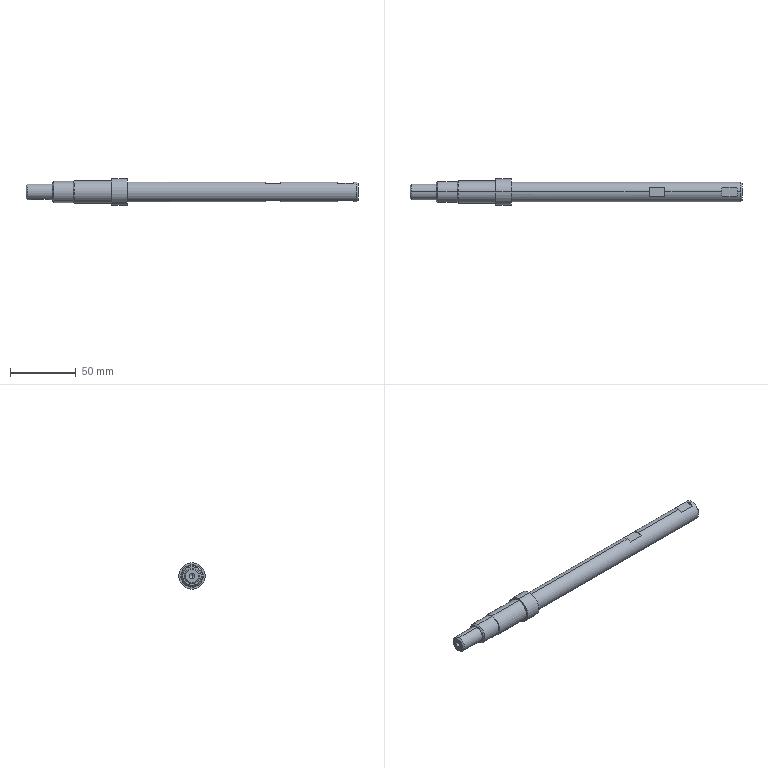Part | STEP file | MT-COMBO-119-S046 | 1 solid | 49 faces | box 252 x 20 x 20 mm | volume 45952 mm3 | plane 20 | cylinder 17 | cone 12 | commonest cylinder face diameters 4.2 x4 4 x3 12 x2 15 x2 16 x2 17 x2
STEP:
#1=CARTESIAN_POINT('',(-216.,0.,-8.));
#2=VERTEX_POINT('',#1);
#3=CARTESIAN_POINT('',(-216.,0.,8.));
#4=VERTEX_POINT('',#3);
#5=CARTESIAN_POINT('',(-216.,0.,0.));
#6=DIRECTION('',(1.,0.,0.));
#7=DIRECTION('',(0.,0.,-1.));
#8=AXIS2_PLACEMENT_3D('',#5,#6,#7);
#9=CIRCLE('',#8,8.);
#10=EDGE_CURVE('',#2,#4,#9,.T.);
#11=ORIENTED_EDGE('',*,*,#10,.T.);
#12=CARTESIAN_POINT('',(-215.5,0.,8.5));
#13=VERTEX_POINT('',#12);
#14=CARTESIAN_POINT('',(-215.5,0.,8.5));
#15=DIRECTION('',(0.7071,0.,0.7071));
#16=VECTOR('',#15,1000.);
#17=LINE('',#14,#16);
#18=EDGE_CURVE('',#4,#13,#17,.T.);
#19=ORIENTED_EDGE('',*,*,#18,.T.);
#20=CARTESIAN_POINT('',(-215.5,0.,-8.5));
#21=VERTEX_POINT('',#20);
#22=CARTESIAN_POINT('',(-215.5,0.,0.));
#23=DIRECTION('',(1.,0.,0.));
#24=DIRECTION('',(0.,0.,1.));
#25=AXIS2_PLACEMENT_3D('',#22,#23,#24);
#26=CIRCLE('',#25,8.5);
#27=EDGE_CURVE('',#21,#13,#26,.T.);
#28=ORIENTED_EDGE('',*,*,#27,.F.);
#29=CARTESIAN_POINT('',(-215.5,0.,-8.5));
#30=DIRECTION('',(0.7071,0.,-0.7071));
#31=VECTOR('',#30,1000.);
#32=LINE('',#29,#31);
#33=EDGE_CURVE('',#2,#21,#32,.T.);
#34=ORIENTED_EDGE('',*,*,#33,.F.);
#35=EDGE_LOOP('',(#11,#19,#28,#34));
#36=FACE_OUTER_BOUND('',#35,.T.);
#37=CARTESIAN_POINT('',(-215.5,0.,0.));
#38=DIRECTION('',(1.,0.,0.));
#39=DIRECTION('',(0.,0.,-1.));
#40=AXIS2_PLACEMENT_3D('',#37,#38,#39);
#41=CONICAL_SURFACE('',#40,8.5,0.7854);
#42=ADVANCED_FACE('',(#36),#41,.T.);
#43=CARTESIAN_POINT('',(-232.,0.,7.));
#44=VERTEX_POINT('',#43);
#45=CARTESIAN_POINT('',(-232.,0.,-7.));
#46=VERTEX_POINT('',#45);
#47=CARTESIAN_POINT('',(-232.,0.,0.));
#48=DIRECTION('',(-1.,0.,0.));
#49=DIRECTION('',(0.,0.,1.));
#50=AXIS2_PLACEMENT_3D('',#47,#48,#49);
#51=CIRCLE('',#50,7.);
#52=EDGE_CURVE('',#44,#46,#51,.T.);
#53=ORIENTED_EDGE('',*,*,#52,.F.);
#54=CARTESIAN_POINT('',(-231.,0.,8.));
#55=VERTEX_POINT('',#54);
#56=CARTESIAN_POINT('',(-231.,0.,8.));
#57=DIRECTION('',(0.7071,0.,0.7071));
#58=VECTOR('',#57,1000.);
#59=LINE('',#56,#58);
#60=EDGE_CURVE('',#44,#55,#59,.T.);
#61=ORIENTED_EDGE('',*,*,#60,.T.);
#62=CARTESIAN_POINT('',(-231.,0.,-8.));
#63=VERTEX_POINT('',#62);
#64=CARTESIAN_POINT('',(-231.,0.,0.));
#65=DIRECTION('',(1.,0.,0.));
#66=DIRECTION('',(0.,0.,1.));
#67=AXIS2_PLACEMENT_3D('',#64,#65,#66);
#68=CIRCLE('',#67,8.);
#69=EDGE_CURVE('',#63,#55,#68,.T.);
#70=ORIENTED_EDGE('',*,*,#69,.F.);
#71=CARTESIAN_POINT('',(-231.,0.,-8.));
#72=DIRECTION('',(0.7071,0.,-0.7071));
#73=VECTOR('',#72,1000.);
#74=LINE('',#71,#73);
#75=EDGE_CURVE('',#46,#63,#74,.T.);
#76=ORIENTED_EDGE('',*,*,#75,.F.);
#77=EDGE_LOOP('',(#53,#61,#70,#76));
#78=FACE_OUTER_BOUND('',#77,.T.);
#79=CARTESIAN_POINT('',(-231.,0.,0.));
#80=DIRECTION('',(1.,0.,0.));
#81=DIRECTION('',(0.,0.,-1.));
#82=AXIS2_PLACEMENT_3D('',#79,#80,#81);
#83=CONICAL_SURFACE('',#82,8.,0.7854);
#84=ADVANCED_FACE('',(#78),#83,.T.);
#85=CARTESIAN_POINT('',(-236.,2.,-5.657));
#86=VERTEX_POINT('',#85);
#87=CARTESIAN_POINT('',(-234.,0.,-6.));
#88=VERTEX_POINT('',#87);
#89=CARTESIAN_POINT('',(-236.,2.,-5.657));
#90=CARTESIAN_POINT('',(-235.867,2.,-5.657));
#91=CARTESIAN_POINT('',(-235.736,1.987,-5.662));
#92=CARTESIAN_POINT('',(-235.479,1.935,-5.679));
#93=CARTESIAN_POINT('',(-235.351,1.896,-5.693));
#94=CARTESIAN_POINT('',(-235.11,1.796,-5.725));
#95=CARTESIAN_POINT('',(-234.995,1.734,-5.744));
#96=CARTESIAN_POINT('',(-234.779,1.589,-5.786));
#97=CARTESIAN_POINT('',(-234.677,1.505,-5.809));
#98=CARTESIAN_POINT('',(-234.402,1.23,-5.876));
#99=CARTESIAN_POINT('',(-234.253,1.009,-5.92));
#100=CARTESIAN_POINT('',(-234.103,0.648,-5.966));
#101=CARTESIAN_POINT('',(-234.065,0.5209,-5.979));
#102=CARTESIAN_POINT('',(-234.013,0.2621,-5.996));
#103=CARTESIAN_POINT('',(-234.,0.1316,-6.));
#104=CARTESIAN_POINT('',(-234.,0.,-6.));
#105=B_SPLINE_CURVE_WITH_KNOTS('',3,(#89,#90,#91,#92,#93,#94,#95,#96,#97,#98,#99,#100,#101,#102,#103,#104),.UNSPECIFIED.,.F.,.F.,(4,2,2,2,2,2,2,4),(0.,0.0003937,0.0007875,0.001181,0.001575,0.002362,0.002756,0.00315),.UNSPECIFIED.);
#106=EDGE_CURVE('',#86,#88,#105,.T.);
#107=ORIENTED_EDGE('',*,*,#106,.T.);
#108=CARTESIAN_POINT('',(-234.,0.,-3.5));
#109=VERTEX_POINT('',#108);
#110=CARTESIAN_POINT('',(-234.,0.,-10.));
#111=DIRECTION('',(0.,0.,1.));
#112=VECTOR('',#111,1000.);
#113=LINE('',#110,#112);
#114=EDGE_CURVE('',#88,#109,#113,.T.);
#115=ORIENTED_EDGE('',*,*,#114,.T.);
#116=CARTESIAN_POINT('',(-236.,2.,-3.5));
#117=VERTEX_POINT('',#116);
#118=CARTESIAN_POINT('',(-236.,0.,-3.5));
#119=DIRECTION('',(0.,0.,1.));
#120=DIRECTION('',(1.,0.,0.));
#121=AXIS2_PLACEMENT_3D('',#118,#119,#120);
#122=CIRCLE('',#121,2.);
#123=EDGE_CURVE('',#109,#117,#122,.T.);
#124=ORIENTED_EDGE('',*,*,#123,.T.);
#125=CARTESIAN_POINT('',(-236.,2.,-10.));
#126=DIRECTION('',(0.,0.,1.));
#127=VECTOR('',#126,1000.);
#128=LINE('',#125,#127);
#129=EDGE_CURVE('',#86,#117,#128,.T.);
#130=ORIENTED_EDGE('',*,*,#129,.F.);
#131=EDGE_LOOP('',(#107,#115,#124,#130));
#132=FACE_OUTER_BOUND('',#131,.T.);
#133=CARTESIAN_POINT('',(-236.,0.,-10.));
#134=DIRECTION('',(0.,0.,1.));
#135=DIRECTION('',(1.,0.,0.));
#136=AXIS2_PLACEMENT_3D('',#133,#134,#135);
#137=CYLINDRICAL_SURFACE('',#136,2.);
#138=ADVANCED_FACE('',(#132),#137,.F.);
#139=CARTESIAN_POINT('',(0.,0.,-6.5));
#140=VERTEX_POINT('',#139);
#141=CARTESIAN_POINT('',(0.,0.,6.5));
#142=VERTEX_POINT('',#141);
#143=CARTESIAN_POINT('',(0.,0.,0.));
#144=DIRECTION('',(1.,0.,0.));
#145=DIRECTION('',(0.,0.,-1.));
#146=AXIS2_PLACEMENT_3D('',#143,#144,#145);
#147=CIRCLE('',#146,6.5);
#148=EDGE_CURVE('',#140,#142,#147,.T.);
#149=ORIENTED_EDGE('',*,*,#148,.F.);
#150=CARTESIAN_POINT('',(-1.,0.,-7.5));
#151=VERTEX_POINT('',#150);
#152=CARTESIAN_POINT('',(0.,0.,-6.5));
#153=DIRECTION('',(-0.7071,0.,-0.7071));
#154=VECTOR('',#153,1000.);
#155=LINE('',#152,#154);
#156=EDGE_CURVE('',#140,#151,#155,.T.);
#157=ORIENTED_EDGE('',*,*,#156,.T.);
#158=CARTESIAN_POINT('',(-1.,0.,7.5));
#159=VERTEX_POINT('',#158);
#160=CARTESIAN_POINT('',(-1.,0.,0.));
#161=DIRECTION('',(-1.,0.,0.));
#162=DIRECTION('',(0.,0.,-1.));
#163=AXIS2_PLACEMENT_3D('',#160,#161,#162);
#164=CIRCLE('',#163,7.5);
#165=EDGE_CURVE('',#159,#151,#164,.T.);
#166=ORIENTED_EDGE('',*,*,#165,.F.);
#167=CARTESIAN_POINT('',(0.,0.,6.5));
#168=DIRECTION('',(-0.7071,0.,0.7071));
#169=VECTOR('',#168,1000.);
#170=LINE('',#167,#169);
#171=EDGE_CURVE('',#142,#159,#170,.T.);
#172=ORIENTED_EDGE('',*,*,#171,.F.);
#173=EDGE_LOOP('',(#149,#157,#166,#172));
#174=FACE_OUTER_BOUND('',#173,.T.);
#175=CARTESIAN_POINT('',(0.,0.,0.));
#176=DIRECTION('',(-1.,0.,0.));
#177=DIRECTION('',(0.,0.,1.));
#178=AXIS2_PLACEMENT_3D('',#175,#176,#177);
#179=CONICAL_SURFACE('',#178,6.5,0.7854);
#180=ADVANCED_FACE('',(#174),#179,.T.);
#181=CARTESIAN_POINT('',(-252.,0.,5.));
#182=VERTEX_POINT('',#181);
#183=CARTESIAN_POINT('',(-252.,0.,-5.));
#184=VERTEX_POINT('',#183);
#185=CARTESIAN_POINT('',(-252.,0.,0.));
#186=DIRECTION('',(-1.,0.,0.));
#187=DIRECTION('',(0.,0.,1.));
#188=AXIS2_PLACEMENT_3D('',#185,#186,#187);
#189=CIRCLE('',#188,5.);
#190=EDGE_CURVE('',#182,#184,#189,.T.);
#191=ORIENTED_EDGE('',*,*,#190,.F.);
#192=CARTESIAN_POINT('',(-251.,0.,6.));
#193=VERTEX_POINT('',#192);
#194=CARTESIAN_POINT('',(-251.,0.,6.));
#195=DIRECTION('',(0.7071,0.,0.7071));
#196=VECTOR('',#195,1000.);
#197=LINE('',#194,#196);
#198=EDGE_CURVE('',#182,#193,#197,.T.);
#199=ORIENTED_EDGE('',*,*,#198,.T.);
#200=CARTESIAN_POINT('',(-251.,0.,-6.));
#201=VERTEX_POINT('',#200);
#202=CARTESIAN_POINT('',(-251.,0.,0.));
#203=DIRECTION('',(1.,0.,0.));
#204=DIRECTION('',(0.,0.,1.));
#205=AXIS2_PLACEMENT_3D('',#202,#203,#204);
#206=CIRCLE('',#205,6.);
#207=EDGE_CURVE('',#201,#193,#206,.T.);
#208=ORIENTED_EDGE('',*,*,#207,.F.);
#209=CARTESIAN_POINT('',(-251.,0.,-6.));
#210=DIRECTION('',(0.7071,0.,-0.7071));
#211=VECTOR('',#210,1000.);
#212=LINE('',#209,#211);
#213=EDGE_CURVE('',#184,#201,#212,.T.);
#214=ORIENTED_EDGE('',*,*,#213,.F.);
#215=EDGE_LOOP('',(#191,#199,#208,#214));
#216=FACE_OUTER_BOUND('',#215,.T.);
#217=CARTESIAN_POINT('',(-251.,0.,0.));
#218=DIRECTION('',(1.,0.,0.));
#219=DIRECTION('',(0.,0.,-1.));
#220=AXIS2_PLACEMENT_3D('',#217,#218,#219);
#221=CONICAL_SURFACE('',#220,6.,0.7854);
#222=ADVANCED_FACE('',(#216),#221,.T.);
#223=CARTESIAN_POINT('',(-239.6,0.,-2.1));
#224=VERTEX_POINT('',#223);
#225=CARTESIAN_POINT('',(-239.6,0.,2.1));
#226=VERTEX_POINT('',#225);
#227=CARTESIAN_POINT('',(-239.6,0.,0.));
#228=DIRECTION('',(-1.,0.,0.));
#229=DIRECTION('',(0.,0.,1.));
#230=AXIS2_PLACEMENT_3D('',#227,#228,#229);
#231=CIRCLE('',#230,2.1);
#232=EDGE_CURVE('',#224,#226,#231,.T.);
#233=ORIENTED_EDGE('',*,*,#232,.F.);
#234=CARTESIAN_POINT('',(-252.,0.,-2.1));
#235=VERTEX_POINT('',#234);
#236=CARTESIAN_POINT('',(-252.,0.,-2.1));
#237=DIRECTION('',(-1.,0.,0.));
#238=VECTOR('',#237,1000.);
#239=LINE('',#236,#238);
#240=EDGE_CURVE('',#224,#235,#239,.T.);
#241=ORIENTED_EDGE('',*,*,#240,.T.);
#242=CARTESIAN_POINT('',(-252.,0.,2.1));
#243=VERTEX_POINT('',#242);
#244=CARTESIAN_POINT('',(-252.,0.,0.));
#245=DIRECTION('',(-1.,0.,0.));
#246=DIRECTION('',(0.,0.,1.));
#247=AXIS2_PLACEMENT_3D('',#244,#245,#246);
#248=CIRCLE('',#247,2.1);
#249=EDGE_CURVE('',#235,#243,#248,.T.);
#250=ORIENTED_EDGE('',*,*,#249,.T.);
#251=CARTESIAN_POINT('',(-252.,0.,2.1));
#252=DIRECTION('',(-1.,0.,0.));
#253=VECTOR('',#252,1000.);
#254=LINE('',#251,#253);
#255=EDGE_CURVE('',#226,#243,#254,.T.);
#256=ORIENTED_EDGE('',*,*,#255,.F.);
#257=EDGE_LOOP('',(#233,#241,#250,#256));
#258=FACE_OUTER_BOUND('',#257,.T.);
#259=CARTESIAN_POINT('',(-252.,0.,0.));
#260=DIRECTION('',(-1.,0.,0.));
#261=DIRECTION('',(0.,0.,1.));
#262=AXIS2_PLACEMENT_3D('',#259,#260,#261);
#263=CYLINDRICAL_SURFACE('',#262,2.1);
#264=ADVANCED_FACE('',(#258),#263,.F.);
#265=CARTESIAN_POINT('',(-238.338,0.,0.));
#266=VERTEX_POINT('',#265);
#267=CARTESIAN_POINT('',(-239.6,0.,2.1));
#268=DIRECTION('',(-0.515,0.,0.8572));
#269=VECTOR('',#268,1000.);
#270=LINE('',#267,#269);
#271=EDGE_CURVE('',#266,#226,#270,.T.);
#272=ORIENTED_EDGE('',*,*,#271,.F.);
#273=CARTESIAN_POINT('',(-239.6,0.,-2.1));
#274=DIRECTION('',(-0.515,0.,-0.8572));
#275=VECTOR('',#274,1000.);
#276=LINE('',#273,#275);
#277=EDGE_CURVE('',#266,#224,#276,.T.);
#278=ORIENTED_EDGE('',*,*,#277,.T.);
#279=ORIENTED_EDGE('',*,*,#232,.T.);
#280=EDGE_LOOP('',(#272,#278,#279));
#281=FACE_OUTER_BOUND('',#280,.T.);
#282=CARTESIAN_POINT('',(-239.6,0.,0.));
#283=DIRECTION('',(-1.,0.,0.));
#284=DIRECTION('',(0.,0.,1.));
#285=AXIS2_PLACEMENT_3D('',#282,#283,#284);
#286=CONICAL_SURFACE('',#285,2.1,1.03);
#287=ADVANCED_FACE('',(#281),#286,.F.);
#288=CARTESIAN_POINT('',(-12.4,0.,2.1));
#289=VERTEX_POINT('',#288);
#290=CARTESIAN_POINT('',(-12.4,0.,-2.1));
#291=VERTEX_POINT('',#290);
#292=CARTESIAN_POINT('',(-12.4,0.,0.));
#293=DIRECTION('',(1.,0.,0.));
#294=DIRECTION('',(0.,0.,-1.));
#295=AXIS2_PLACEMENT_3D('',#292,#293,#294);
#296=CIRCLE('',#295,2.1);
#297=EDGE_CURVE('',#289,#291,#296,.T.);
#298=ORIENTED_EDGE('',*,*,#297,.F.);
#299=CARTESIAN_POINT('',(0.,0.,2.1));
#300=VERTEX_POINT('',#299);
#301=CARTESIAN_POINT('',(0.,0.,2.1));
#302=DIRECTION('',(1.,0.,0.));
#303=VECTOR('',#302,1000.);
#304=LINE('',#301,#303);
#305=EDGE_CURVE('',#289,#300,#304,.T.);
#306=ORIENTED_EDGE('',*,*,#305,.T.);
#307=CARTESIAN_POINT('',(0.,0.,-2.1));
#308=VERTEX_POINT('',#307);
#309=CARTESIAN_POINT('',(0.,0.,0.));
#310=DIRECTION('',(1.,0.,0.));
#311=DIRECTION('',(0.,0.,-1.));
#312=AXIS2_PLACEMENT_3D('',#309,#310,#311);
#313=CIRCLE('',#312,2.1);
#314=EDGE_CURVE('',#300,#308,#313,.T.);
#315=ORIENTED_EDGE('',*,*,#314,.T.);
#316=CARTESIAN_POINT('',(0.,0.,-2.1));
#317=DIRECTION('',(1.,0.,0.));
#318=VECTOR('',#317,1000.);
#319=LINE('',#316,#318);
#320=EDGE_CURVE('',#291,#308,#319,.T.);
#321=ORIENTED_EDGE('',*,*,#320,.F.);
#322=EDGE_LOOP('',(#298,#306,#315,#321));
#323=FACE_OUTER_BOUND('',#322,.T.);
#324=CARTESIAN_POINT('',(0.,0.,0.));
#325=DIRECTION('',(1.,0.,0.));
#326=DIRECTION('',(0.,0.,-1.));
#327=AXIS2_PLACEMENT_3D('',#324,#325,#326);
#328=CYLINDRICAL_SURFACE('',#327,2.1);
#329=ADVANCED_FACE('',(#323),#328,.F.);
#330=CARTESIAN_POINT('',(-13.662,0.,0.));
#331=VERTEX_POINT('',#330);
#332=CARTESIAN_POINT('',(-12.4,0.,-2.1));
#333=DIRECTION('',(0.515,0.,-0.8572));
#334=VECTOR('',#333,1000.);
#335=LINE('',#332,#334);
#336=EDGE_CURVE('',#331,#291,#335,.T.);
#337=ORIENTED_EDGE('',*,*,#336,.F.);
#338=CARTESIAN_POINT('',(-12.4,0.,2.1));
#339=DIRECTION('',(0.515,0.,0.8572));
#340=VECTOR('',#339,1000.);
#341=LINE('',#338,#340);
#342=EDGE_CURVE('',#331,#289,#341,.T.);
#343=ORIENTED_EDGE('',*,*,#342,.T.);
#344=ORIENTED_EDGE('',*,*,#297,.T.);
#345=EDGE_LOOP('',(#337,#343,#344));
#346=FACE_OUTER_BOUND('',#345,.T.);
#347=CARTESIAN_POINT('',(-12.4,0.,0.));
#348=DIRECTION('',(1.,0.,0.));
#349=DIRECTION('',(0.,0.,-1.));
#350=AXIS2_PLACEMENT_3D('',#347,#348,#349);
#351=CONICAL_SURFACE('',#350,2.1,1.03);
#352=ADVANCED_FACE('',(#346),#351,.F.);
#353=ORIENTED_EDGE('',*,*,#207,.T.);
#354=CARTESIAN_POINT('',(-232.,0.,6.));
#355=VERTEX_POINT('',#354);
#356=CARTESIAN_POINT('',(0.,0.,6.));
#357=DIRECTION('',(1.,0.,0.));
#358=VECTOR('',#357,1000.);
#359=LINE('',#356,#358);
#360=EDGE_CURVE('',#193,#355,#359,.T.);
#361=ORIENTED_EDGE('',*,*,#360,.T.);
#362=CARTESIAN_POINT('',(-232.,0.,-6.));
#363=VERTEX_POINT('',#362);
#364=CARTESIAN_POINT('',(-232.,0.,0.));
#365=DIRECTION('',(1.,0.,0.));
#366=DIRECTION('',(0.,0.,-1.));
#367=AXIS2_PLACEMENT_3D('',#364,#365,#366);
#368=CIRCLE('',#367,6.);
#369=EDGE_CURVE('',#363,#355,#368,.T.);
#370=ORIENTED_EDGE('',*,*,#369,.F.);
#371=CARTESIAN_POINT('',(0.,0.,-6.));
#372=DIRECTION('',(1.,0.,0.));
#373=VECTOR('',#372,1000.);
#374=LINE('',#371,#373);
#375=EDGE_CURVE('',#88,#363,#374,.T.);
#376=ORIENTED_EDGE('',*,*,#375,.F.);
#377=ORIENTED_EDGE('',*,*,#106,.F.);
#378=CARTESIAN_POINT('',(-247.,2.,-5.657));
#379=VERTEX_POINT('',#378);
#380=CARTESIAN_POINT('',(0.,2.,-5.657));
#381=DIRECTION('',(1.,0.,0.));
#382=VECTOR('',#381,1000.);
#383=LINE('',#380,#382);
#384=EDGE_CURVE('',#379,#86,#383,.T.);
#385=ORIENTED_EDGE('',*,*,#384,.F.);
#386=CARTESIAN_POINT('',(-249.,0.,-6.));
#387=VERTEX_POINT('',#386);
#388=CARTESIAN_POINT('',(-249.,0.,-6.));
#389=CARTESIAN_POINT('',(-249.,0.1314,-6.));
#390=CARTESIAN_POINT('',(-248.987,0.2649,-5.996));
#391=CARTESIAN_POINT('',(-248.935,0.5219,-5.979));
#392=CARTESIAN_POINT('',(-248.897,0.647,-5.966));
#393=CARTESIAN_POINT('',(-248.796,0.8902,-5.935));
#394=CARTESIAN_POINT('',(-248.734,1.006,-5.916));
#395=CARTESIAN_POINT('',(-248.589,1.221,-5.875));
#396=CARTESIAN_POINT('',(-248.506,1.323,-5.853));
#397=CARTESIAN_POINT('',(-248.322,1.507,-5.809));
#398=CARTESIAN_POINT('',(-248.222,1.589,-5.786));
#399=CARTESIAN_POINT('',(-248.006,1.733,-5.745));
#400=CARTESIAN_POINT('',(-247.889,1.796,-5.725));
#401=CARTESIAN_POINT('',(-247.529,1.946,-5.677));
#402=CARTESIAN_POINT('',(-247.266,2.,-5.657));
#403=CARTESIAN_POINT('',(-247.,2.,-5.657));
#404=B_SPLINE_CURVE_WITH_KNOTS('',3,(#388,#389,#390,#391,#392,#393,#394,#395,#396,#397,#398,#399,#400,#401,#402,#403),.UNSPECIFIED.,.F.,.F.,(4,2,2,2,2,2,2,4),(0.00315,0.003543,0.003936,0.00433,0.004723,0.005116,0.005509,0.006296),.UNSPECIFIED.);
#405=EDGE_CURVE('',#387,#379,#404,.T.);
#406=ORIENTED_EDGE('',*,*,#405,.F.);
#407=CARTESIAN_POINT('',(0.,0.,-6.));
#408=DIRECTION('',(1.,0.,0.));
#409=VECTOR('',#408,1000.);
#410=LINE('',#407,#409);
#411=EDGE_CURVE('',#201,#387,#410,.T.);
#412=ORIENTED_EDGE('',*,*,#411,.F.);
#413=EDGE_LOOP('',(#353,#361,#370,#376,#377,#385,#406,#412));
#414=FACE_OUTER_BOUND('',#413,.T.);
#415=CARTESIAN_POINT('',(0.,0.,0.));
#416=DIRECTION('',(1.,0.,0.));
#417=DIRECTION('',(0.,0.,-1.));
#418=AXIS2_PLACEMENT_3D('',#415,#416,#417);
#419=CYLINDRICAL_SURFACE('',#418,6.);
#420=ADVANCED_FACE('',(#414),#419,.T.);
#421=ORIENTED_EDGE('',*,*,#69,.T.);
#422=CARTESIAN_POINT('',(0.,0.,8.));
#423=DIRECTION('',(1.,0.,0.));
#424=VECTOR('',#423,1000.);
#425=LINE('',#422,#424);
#426=EDGE_CURVE('',#55,#4,#425,.T.);
#427=ORIENTED_EDGE('',*,*,#426,.T.);
#428=ORIENTED_EDGE('',*,*,#10,.F.);
#429=CARTESIAN_POINT('',(0.,0.,-8.));
#430=DIRECTION('',(1.,0.,0.));
#431=VECTOR('',#430,1000.);
#432=LINE('',#429,#431);
#433=EDGE_CURVE('',#63,#2,#432,.T.);
#434=ORIENTED_EDGE('',*,*,#433,.F.);
#435=EDGE_LOOP('',(#421,#427,#428,#434));
#436=FACE_OUTER_BOUND('',#435,.T.);
#437=CARTESIAN_POINT('',(0.,0.,0.));
#438=DIRECTION('',(1.,0.,0.));
#439=DIRECTION('',(0.,0.,-1.));
#440=AXIS2_PLACEMENT_3D('',#437,#438,#439);
#441=CYLINDRICAL_SURFACE('',#440,8.);
#442=ADVANCED_FACE('',(#436),#441,.T.);
#443=ORIENTED_EDGE('',*,*,#27,.T.);
#444=CARTESIAN_POINT('',(-187.,0.,8.5));
#445=VERTEX_POINT('',#444);
#446=CARTESIAN_POINT('',(0.,0.,8.5));
#447=DIRECTION('',(1.,0.,0.));
#448=VECTOR('',#447,1000.);
#449=LINE('',#446,#448);
#450=EDGE_CURVE('',#13,#445,#449,.T.);
#451=ORIENTED_EDGE('',*,*,#450,.T.);
#452=CARTESIAN_POINT('',(-187.,0.,-8.5));
#453=VERTEX_POINT('',#452);
#454=CARTESIAN_POINT('',(-187.,0.,0.));
#455=DIRECTION('',(1.,0.,0.));
#456=DIRECTION('',(0.,0.,-1.));
#457=AXIS2_PLACEMENT_3D('',#454,#455,#456);
#458=CIRCLE('',#457,8.5);
#459=EDGE_CURVE('',#453,#445,#458,.T.);
#460=ORIENTED_EDGE('',*,*,#459,.F.);
#461=CARTESIAN_POINT('',(0.,0.,-8.5));
#462=DIRECTION('',(1.,0.,0.));
#463=VECTOR('',#462,1000.);
#464=LINE('',#461,#463);
#465=EDGE_CURVE('',#21,#453,#464,.T.);
#466=ORIENTED_EDGE('',*,*,#465,.F.);
#467=EDGE_LOOP('',(#443,#451,#460,#466));
#468=FACE_OUTER_BOUND('',#467,.T.);
#469=CARTESIAN_POINT('',(0.,0.,0.));
#470=DIRECTION('',(1.,0.,0.));
#471=DIRECTION('',(0.,0.,-1.));
#472=AXIS2_PLACEMENT_3D('',#469,#470,#471);
#473=CYLINDRICAL_SURFACE('',#472,8.5);
#474=ADVANCED_FACE('',(#468),#473,.T.);
#475=CARTESIAN_POINT('',(-187.,0.,-10.));
#476=VERTEX_POINT('',#475);
#477=CARTESIAN_POINT('',(-187.,0.,10.));
#478=VERTEX_POINT('',#477);
#479=CARTESIAN_POINT('',(-187.,0.,0.));
#480=DIRECTION('',(1.,0.,0.));
#481=DIRECTION('',(0.,0.,-1.));
#482=AXIS2_PLACEMENT_3D('',#479,#480,#481);
#483=CIRCLE('',#482,10.);
#484=EDGE_CURVE('',#476,#478,#483,.T.);
#485=ORIENTED_EDGE('',*,*,#484,.T.);
#486=CARTESIAN_POINT('',(-175.,0.,10.));
#487=VERTEX_POINT('',#486);
#488=CARTESIAN_POINT('',(0.,0.,10.));
#489=DIRECTION('',(1.,0.,0.));
#490=VECTOR('',#489,1000.);
#491=LINE('',#488,#490);
#492=EDGE_CURVE('',#478,#487,#491,.T.);
#493=ORIENTED_EDGE('',*,*,#492,.T.);
#494=CARTESIAN_POINT('',(-175.,0.,-10.));
#495=VERTEX_POINT('',#494);
#496=CARTESIAN_POINT('',(-175.,0.,0.));
#497=DIRECTION('',(1.,0.,0.));
#498=DIRECTION('',(0.,0.,-1.));
#499=AXIS2_PLACEMENT_3D('',#496,#497,#498);
#500=CIRCLE('',#499,10.);
#501=EDGE_CURVE('',#495,#487,#500,.T.);
#502=ORIENTED_EDGE('',*,*,#501,.F.);
#503=CARTESIAN_POINT('',(0.,0.,-10.));
#504=DIRECTION('',(1.,0.,0.));
#505=VECTOR('',#504,1000.);
#506=LINE('',#503,#505);
#507=EDGE_CURVE('',#476,#495,#506,.T.);
#508=ORIENTED_EDGE('',*,*,#507,.F.);
#509=EDGE_LOOP('',(#485,#493,#502,#508));
#510=FACE_OUTER_BOUND('',#509,.T.);
#511=CARTESIAN_POINT('',(0.,0.,0.));
#512=DIRECTION('',(1.,0.,0.));
#513=DIRECTION('',(0.,0.,-1.));
#514=AXIS2_PLACEMENT_3D('',#511,#512,#513);
#515=CYLINDRICAL_SURFACE('',#514,10.);
#516=ADVANCED_FACE('',(#510),#515,.T.);
#517=CARTESIAN_POINT('',(-175.,0.,-7.5));
#518=VERTEX_POINT('',#517);
#519=CARTESIAN_POINT('',(-175.,0.,7.5));
#520=VERTEX_POINT('',#519);
#521=CARTESIAN_POINT('',(-175.,0.,0.));
#522=DIRECTION('',(1.,0.,0.));
#523=DIRECTION('',(0.,0.,-1.));
#524=AXIS2_PLACEMENT_3D('',#521,#522,#523);
#525=CIRCLE('',#524,7.5);
#526=EDGE_CURVE('',#518,#520,#525,.T.);
#527=ORIENTED_EDGE('',*,*,#526,.T.);
#528=CARTESIAN_POINT('',(-70.5,0.,7.5));
#529=VERTEX_POINT('',#528);
#530=CARTESIAN_POINT('',(0.,0.,7.5));
#531=DIRECTION('',(1.,0.,0.));
#532=VECTOR('',#531,1000.);
#533=LINE('',#530,#532);
#534=EDGE_CURVE('',#520,#529,#533,.T.);
#535=ORIENTED_EDGE('',*,*,#534,.T.);
#536=CARTESIAN_POINT('',(-70.5,3.742,6.5));
#537=VERTEX_POINT('',#536);
#538=CARTESIAN_POINT('',(-70.5,0.,0.));
#539=DIRECTION('',(1.,0.,0.));
#540=DIRECTION('',(0.,0.,1.));
#541=AXIS2_PLACEMENT_3D('',#538,#539,#540);
#542=CIRCLE('',#541,7.5);
#543=EDGE_CURVE('',#537,#529,#542,.T.);
#544=ORIENTED_EDGE('',*,*,#543,.F.);
#545=CARTESIAN_POINT('',(-58.5,3.742,6.5));
#546=VERTEX_POINT('',#545);
#547=CARTESIAN_POINT('',(0.,3.742,6.5));
#548=DIRECTION('',(-1.,0.,0.));
#549=VECTOR('',#548,1000.);
#550=LINE('',#547,#549);
#551=EDGE_CURVE('',#546,#537,#550,.T.);
#552=ORIENTED_EDGE('',*,*,#551,.F.);
#553=CARTESIAN_POINT('',(-58.5,0.,7.5));
#554=VERTEX_POINT('',#553);
#555=CARTESIAN_POINT('',(-58.5,0.,0.));
#556=DIRECTION('',(-1.,0.,0.));
#557=DIRECTION('',(0.,0.,-1.));
#558=AXIS2_PLACEMENT_3D('',#555,#556,#557);
#559=CIRCLE('',#558,7.5);
#560=EDGE_CURVE('',#554,#546,#559,.T.);
#561=ORIENTED_EDGE('',*,*,#560,.F.);
#562=CARTESIAN_POINT('',(-15.5,0.,7.5));
#563=VERTEX_POINT('',#562);
#564=CARTESIAN_POINT('',(0.,0.,7.5));
#565=DIRECTION('',(1.,0.,0.));
#566=VECTOR('',#565,1000.);
#567=LINE('',#564,#566);
#568=EDGE_CURVE('',#554,#563,#567,.T.);
#569=ORIENTED_EDGE('',*,*,#568,.T.);
#570=CARTESIAN_POINT('',(-15.5,3.742,6.5));
#571=VERTEX_POINT('',#570);
#572=CARTESIAN_POINT('',(-15.5,0.,0.));
#573=DIRECTION('',(1.,0.,0.));
#574=DIRECTION('',(0.,0.,1.));
#575=AXIS2_PLACEMENT_3D('',#572,#573,#574);
#576=CIRCLE('',#575,7.5);
#577=EDGE_CURVE('',#571,#563,#576,.T.);
#578=ORIENTED_EDGE('',*,*,#577,.F.);
#579=CARTESIAN_POINT('',(-3.5,3.742,6.5));
#580=VERTEX_POINT('',#579);
#581=CARTESIAN_POINT('',(0.,3.742,6.5));
#582=DIRECTION('',(-1.,0.,0.));
#583=VECTOR('',#582,1000.);
#584=LINE('',#581,#583);
#585=EDGE_CURVE('',#580,#571,#584,.T.);
#586=ORIENTED_EDGE('',*,*,#585,.F.);
#587=CARTESIAN_POINT('',(-3.5,0.,7.5));
#588=VERTEX_POINT('',#587);
#589=CARTESIAN_POINT('',(-3.5,0.,0.));
#590=DIRECTION('',(-1.,0.,0.));
#591=DIRECTION('',(0.,0.,-1.));
#592=AXIS2_PLACEMENT_3D('',#589,#590,#591);
#593=CIRCLE('',#592,7.5);
#594=EDGE_CURVE('',#588,#580,#593,.T.);
#595=ORIENTED_EDGE('',*,*,#594,.F.);
#596=CARTESIAN_POINT('',(0.,0.,7.5));
#597=DIRECTION('',(1.,0.,0.));
#598=VECTOR('',#597,1000.);
#599=LINE('',#596,#598);
#600=EDGE_CURVE('',#588,#159,#599,.T.);
#601=ORIENTED_EDGE('',*,*,#600,.T.);
#602=ORIENTED_EDGE('',*,*,#165,.T.);
#603=CARTESIAN_POINT('',(-3.5,0.,-7.5));
#604=VERTEX_POINT('',#603);
#605=CARTESIAN_POINT('',(0.,0.,-7.5));
#606=DIRECTION('',(1.,0.,0.));
#607=VECTOR('',#606,1000.);
#608=LINE('',#605,#607);
#609=EDGE_CURVE('',#604,#151,#608,.T.);
#610=ORIENTED_EDGE('',*,*,#609,.F.);
#611=CARTESIAN_POINT('',(-3.5,3.742,-6.5));
#612=VERTEX_POINT('',#611);
#613=CARTESIAN_POINT('',(-3.5,0.,0.));
#614=DIRECTION('',(-1.,0.,0.));
#615=DIRECTION('',(0.,0.,-1.));
#616=AXIS2_PLACEMENT_3D('',#613,#614,#615);
#617=CIRCLE('',#616,7.5);
#618=EDGE_CURVE('',#612,#604,#617,.T.);
#619=ORIENTED_EDGE('',*,*,#618,.F.);
#620=CARTESIAN_POINT('',(-15.5,3.742,-6.5));
#621=VERTEX_POINT('',#620);
#622=CARTESIAN_POINT('',(0.,3.742,-6.5));
#623=DIRECTION('',(1.,0.,0.));
#624=VECTOR('',#623,1000.);
#625=LINE('',#622,#624);
#626=EDGE_CURVE('',#621,#612,#625,.T.);
#627=ORIENTED_EDGE('',*,*,#626,.F.);
#628=CARTESIAN_POINT('',(-15.5,0.,-7.5));
#629=VERTEX_POINT('',#628);
#630=CARTESIAN_POINT('',(-15.5,0.,0.));
#631=DIRECTION('',(1.,0.,0.));
#632=DIRECTION('',(0.,0.,1.));
#633=AXIS2_PLACEMENT_3D('',#630,#631,#632);
#634=CIRCLE('',#633,7.5);
#635=EDGE_CURVE('',#629,#621,#634,.T.);
#636=ORIENTED_EDGE('',*,*,#635,.F.);
#637=CARTESIAN_POINT('',(-58.5,0.,-7.5));
#638=VERTEX_POINT('',#637);
#639=CARTESIAN_POINT('',(0.,0.,-7.5));
#640=DIRECTION('',(1.,0.,0.));
#641=VECTOR('',#640,1000.);
#642=LINE('',#639,#641);
#643=EDGE_CURVE('',#638,#629,#642,.T.);
#644=ORIENTED_EDGE('',*,*,#643,.F.);
#645=CARTESIAN_POINT('',(-58.5,3.742,-6.5));
#646=VERTEX_POINT('',#645);
#647=CARTESIAN_POINT('',(-58.5,0.,0.));
#648=DIRECTION('',(-1.,0.,0.));
#649=DIRECTION('',(0.,0.,-1.));
#650=AXIS2_PLACEMENT_3D('',#647,#648,#649);
#651=CIRCLE('',#650,7.5);
#652=EDGE_CURVE('',#646,#638,#651,.T.);
#653=ORIENTED_EDGE('',*,*,#652,.F.);
#654=CARTESIAN_POINT('',(-70.5,3.742,-6.5));
#655=VERTEX_POINT('',#654);
#656=CARTESIAN_POINT('',(0.,3.742,-6.5));
#657=DIRECTION('',(1.,0.,0.));
#658=VECTOR('',#657,1000.);
#659=LINE('',#656,#658);
#660=EDGE_CURVE('',#655,#646,#659,.T.);
#661=ORIENTED_EDGE('',*,*,#660,.F.);
#662=CARTESIAN_POINT('',(-70.5,0.,-7.5));
#663=VERTEX_POINT('',#662);
#664=CARTESIAN_POINT('',(-70.5,0.,0.));
#665=DIRECTION('',(1.,0.,0.));
#666=DIRECTION('',(0.,0.,1.));
#667=AXIS2_PLACEMENT_3D('',#664,#665,#666);
#668=CIRCLE('',#667,7.5);
#669=EDGE_CURVE('',#663,#655,#668,.T.);
#670=ORIENTED_EDGE('',*,*,#669,.F.);
#671=CARTESIAN_POINT('',(0.,0.,-7.5));
#672=DIRECTION('',(1.,0.,0.));
#673=VECTOR('',#672,1000.);
#674=LINE('',#671,#673);
#675=EDGE_CURVE('',#518,#663,#674,.T.);
#676=ORIENTED_EDGE('',*,*,#675,.F.);
#677=EDGE_LOOP('',(#527,#535,#544,#552,#561,#569,#578,#586,#595,#601,#602,#610,#619,#627,#636,#644,#653,#661,#670,#676));
#678=FACE_OUTER_BOUND('',#677,.T.);
#679=CARTESIAN_POINT('',(0.,0.,0.));
#680=DIRECTION('',(1.,0.,0.));
#681=DIRECTION('',(0.,0.,-1.));
#682=AXIS2_PLACEMENT_3D('',#679,#680,#681);
#683=CYLINDRICAL_SURFACE('',#682,7.5);
#684=ADVANCED_FACE('',(#678),#683,.T.);
#685=CARTESIAN_POINT('',(0.,0.,0.));
#686=DIRECTION('',(1.,0.,0.));
#687=DIRECTION('',(0.,0.,-1.));
#688=AXIS2_PLACEMENT_3D('',#685,#686,#687);
#689=CIRCLE('',#688,6.5);
#690=EDGE_CURVE('',#142,#140,#689,.T.);
#691=ORIENTED_EDGE('',*,*,#690,.T.);
#692=ORIENTED_EDGE('',*,*,#148,.T.);
#693=EDGE_LOOP('',(#691,#692));
#694=FACE_OUTER_BOUND('',#693,.T.);
#695=CARTESIAN_POINT('',(0.,0.,0.));
#696=DIRECTION('',(1.,0.,0.));
#697=DIRECTION('',(0.,0.,-1.));
#698=AXIS2_PLACEMENT_3D('',#695,#696,#697);
#699=CIRCLE('',#698,2.1);
#700=EDGE_CURVE('',#308,#300,#699,.T.);
#701=ORIENTED_EDGE('',*,*,#700,.F.);
#702=ORIENTED_EDGE('',*,*,#314,.F.);
#703=EDGE_LOOP('',(#701,#702));
#704=FACE_BOUND('',#703,.T.);
#705=CARTESIAN_POINT('',(0.,0.,0.));
#706=DIRECTION('',(1.,0.,0.));
#707=DIRECTION('',(0.,0.,-1.));
#708=AXIS2_PLACEMENT_3D('',#705,#706,#707);
#709=PLANE('',#708);
#710=ADVANCED_FACE('',(#694,#704),#709,.T.);
#711=ORIENTED_EDGE('',*,*,#534,.F.);
#712=CARTESIAN_POINT('',(-175.,0.,0.));
#713=DIRECTION('',(1.,0.,0.));
#714=DIRECTION('',(0.,0.,-1.));
#715=AXIS2_PLACEMENT_3D('',#712,#713,#714);
#716=CIRCLE('',#715,7.5);
#717=EDGE_CURVE('',#520,#518,#716,.T.);
#718=ORIENTED_EDGE('',*,*,#717,.T.);
#719=ORIENTED_EDGE('',*,*,#675,.T.);
#720=CARTESIAN_POINT('',(-70.5,-3.742,-6.5));
#721=VERTEX_POINT('',#720);
#722=CARTESIAN_POINT('',(-70.5,0.,0.));
#723=DIRECTION('',(1.,0.,0.));
#724=DIRECTION('',(0.,0.,1.));
#725=AXIS2_PLACEMENT_3D('',#722,#723,#724);
#726=CIRCLE('',#725,7.5);
#727=EDGE_CURVE('',#721,#663,#726,.T.);
#728=ORIENTED_EDGE('',*,*,#727,.F.);
#729=CARTESIAN_POINT('',(-58.5,-3.742,-6.5));
#730=VERTEX_POINT('',#729);
#731=CARTESIAN_POINT('',(0.,-3.742,-6.5));
#732=DIRECTION('',(-1.,0.,0.));
#733=VECTOR('',#732,1000.);
#734=LINE('',#731,#733);
#735=EDGE_CURVE('',#730,#721,#734,.T.);
#736=ORIENTED_EDGE('',*,*,#735,.F.);
#737=CARTESIAN_POINT('',(-58.5,0.,0.));
#738=DIRECTION('',(-1.,0.,0.));
#739=DIRECTION('',(0.,0.,-1.));
#740=AXIS2_PLACEMENT_3D('',#737,#738,#739);
#741=CIRCLE('',#740,7.5);
#742=EDGE_CURVE('',#638,#730,#741,.T.);
#743=ORIENTED_EDGE('',*,*,#742,.F.);
#744=ORIENTED_EDGE('',*,*,#643,.T.);
#745=CARTESIAN_POINT('',(-15.5,-3.742,-6.5));
#746=VERTEX_POINT('',#745);
#747=CARTESIAN_POINT('',(-15.5,0.,0.));
#748=DIRECTION('',(1.,0.,0.));
#749=DIRECTION('',(0.,0.,1.));
#750=AXIS2_PLACEMENT_3D('',#747,#748,#749);
#751=CIRCLE('',#750,7.5);
#752=EDGE_CURVE('',#746,#629,#751,.T.);
#753=ORIENTED_EDGE('',*,*,#752,.F.);
#754=CARTESIAN_POINT('',(-3.5,-3.742,-6.5));
#755=VERTEX_POINT('',#754);
#756=CARTESIAN_POINT('',(0.,-3.742,-6.5));
#757=DIRECTION('',(-1.,0.,0.));
#758=VECTOR('',#757,1000.);
#759=LINE('',#756,#758);
#760=EDGE_CURVE('',#755,#746,#759,.T.);
#761=ORIENTED_EDGE('',*,*,#760,.F.);
#762=CARTESIAN_POINT('',(-3.5,0.,0.));
#763=DIRECTION('',(-1.,0.,0.));
#764=DIRECTION('',(0.,0.,-1.));
#765=AXIS2_PLACEMENT_3D('',#762,#763,#764);
#766=CIRCLE('',#765,7.5);
#767=EDGE_CURVE('',#604,#755,#766,.T.);
#768=ORIENTED_EDGE('',*,*,#767,.F.);
#769=ORIENTED_EDGE('',*,*,#609,.T.);
#770=CARTESIAN_POINT('',(-1.,0.,0.));
#771=DIRECTION('',(-1.,0.,0.));
#772=DIRECTION('',(0.,0.,-1.));
#773=AXIS2_PLACEMENT_3D('',#770,#771,#772);
#774=CIRCLE('',#773,7.5);
#775=EDGE_CURVE('',#151,#159,#774,.T.);
#776=ORIENTED_EDGE('',*,*,#775,.T.);
#777=ORIENTED_EDGE('',*,*,#600,.F.);
#778=CARTESIAN_POINT('',(-3.5,-3.742,6.5));
#779=VERTEX_POINT('',#778);
#780=CARTESIAN_POINT('',(-3.5,0.,0.));
#781=DIRECTION('',(-1.,0.,0.));
#782=DIRECTION('',(0.,0.,-1.));
#783=AXIS2_PLACEMENT_3D('',#780,#781,#782);
#784=CIRCLE('',#783,7.5);
#785=EDGE_CURVE('',#779,#588,#784,.T.);
#786=ORIENTED_EDGE('',*,*,#785,.F.);
#787=CARTESIAN_POINT('',(-15.5,-3.742,6.5));
#788=VERTEX_POINT('',#787);
#789=CARTESIAN_POINT('',(0.,-3.742,6.5));
#790=DIRECTION('',(1.,0.,0.));
#791=VECTOR('',#790,1000.);
#792=LINE('',#789,#791);
#793=EDGE_CURVE('',#788,#779,#792,.T.);
#794=ORIENTED_EDGE('',*,*,#793,.F.);
#795=CARTESIAN_POINT('',(-15.5,0.,0.));
#796=DIRECTION('',(1.,0.,0.));
#797=DIRECTION('',(0.,0.,1.));
#798=AXIS2_PLACEMENT_3D('',#795,#796,#797);
#799=CIRCLE('',#798,7.5);
#800=EDGE_CURVE('',#563,#788,#799,.T.);
#801=ORIENTED_EDGE('',*,*,#800,.F.);
#802=ORIENTED_EDGE('',*,*,#568,.F.);
#803=CARTESIAN_POINT('',(-58.5,-3.742,6.5));
#804=VERTEX_POINT('',#803);
#805=CARTESIAN_POINT('',(-58.5,0.,0.));
#806=DIRECTION('',(-1.,0.,0.));
#807=DIRECTION('',(0.,0.,-1.));
#808=AXIS2_PLACEMENT_3D('',#805,#806,#807);
#809=CIRCLE('',#808,7.5);
#810=EDGE_CURVE('',#804,#554,#809,.T.);
#811=ORIENTED_EDGE('',*,*,#810,.F.);
#812=CARTESIAN_POINT('',(-70.5,-3.742,6.5));
#813=VERTEX_POINT('',#812);
#814=CARTESIAN_POINT('',(0.,-3.742,6.5));
#815=DIRECTION('',(1.,0.,0.));
#816=VECTOR('',#815,1000.);
#817=LINE('',#814,#816);
#818=EDGE_CURVE('',#813,#804,#817,.T.);
#819=ORIENTED_EDGE('',*,*,#818,.F.);
#820=CARTESIAN_POINT('',(-70.5,0.,0.));
#821=DIRECTION('',(1.,0.,0.));
#822=DIRECTION('',(0.,0.,1.));
#823=AXIS2_PLACEMENT_3D('',#820,#821,#822);
#824=CIRCLE('',#823,7.5);
#825=EDGE_CURVE('',#529,#813,#824,.T.);
#826=ORIENTED_EDGE('',*,*,#825,.F.);
#827=EDGE_LOOP('',(#711,#718,#719,#728,#736,#743,#744,#753,#761,#768,#769,#776,#777,#786,#794,#801,#802,#811,#819,#826));
#828=FACE_OUTER_BOUND('',#827,.T.);
#829=CARTESIAN_POINT('',(0.,0.,0.));
#830=DIRECTION('',(1.,0.,0.));
#831=DIRECTION('',(0.,0.,-1.));
#832=AXIS2_PLACEMENT_3D('',#829,#830,#831);
#833=CYLINDRICAL_SURFACE('',#832,7.5);
#834=ADVANCED_FACE('',(#828),#833,.T.);
#835=ORIENTED_EDGE('',*,*,#501,.T.);
#836=CARTESIAN_POINT('',(-175.,0.,0.));
#837=DIRECTION('',(1.,0.,0.));
#838=DIRECTION('',(0.,0.,-1.));
#839=AXIS2_PLACEMENT_3D('',#836,#837,#838);
#840=CIRCLE('',#839,10.);
#841=EDGE_CURVE('',#487,#495,#840,.T.);
#842=ORIENTED_EDGE('',*,*,#841,.T.);
#843=EDGE_LOOP('',(#835,#842));
#844=FACE_OUTER_BOUND('',#843,.T.);
#845=ORIENTED_EDGE('',*,*,#526,.F.);
#846=ORIENTED_EDGE('',*,*,#717,.F.);
#847=EDGE_LOOP('',(#845,#846));
#848=FACE_BOUND('',#847,.T.);
#849=CARTESIAN_POINT('',(-175.,7.5,0.));
#850=DIRECTION('',(1.,0.,0.));
#851=DIRECTION('',(0.,0.,-1.));
#852=AXIS2_PLACEMENT_3D('',#849,#850,#851);
#853=PLANE('',#852);
#854=ADVANCED_FACE('',(#844,#848),#853,.T.);
#855=ORIENTED_EDGE('',*,*,#492,.F.);
#856=CARTESIAN_POINT('',(-187.,0.,0.));
#857=DIRECTION('',(1.,0.,0.));
#858=DIRECTION('',(0.,0.,-1.));
#859=AXIS2_PLACEMENT_3D('',#856,#857,#858);
#860=CIRCLE('',#859,10.);
#861=EDGE_CURVE('',#478,#476,#860,.T.);
#862=ORIENTED_EDGE('',*,*,#861,.T.);
#863=ORIENTED_EDGE('',*,*,#507,.T.);
#864=ORIENTED_EDGE('',*,*,#841,.F.);
#865=EDGE_LOOP('',(#855,#862,#863,#864));
#866=FACE_OUTER_BOUND('',#865,.T.);
#867=CARTESIAN_POINT('',(0.,0.,0.));
#868=DIRECTION('',(1.,0.,0.));
#869=DIRECTION('',(0.,0.,-1.));
#870=AXIS2_PLACEMENT_3D('',#867,#868,#869);
#871=CYLINDRICAL_SURFACE('',#870,10.);
#872=ADVANCED_FACE('',(#866),#871,.T.);
#873=ORIENTED_EDGE('',*,*,#459,.T.);
#874=CARTESIAN_POINT('',(-187.,0.,0.));
#875=DIRECTION('',(1.,0.,0.));
#876=DIRECTION('',(0.,0.,-1.));
#877=AXIS2_PLACEMENT_3D('',#874,#875,#876);
#878=CIRCLE('',#877,8.5);
#879=EDGE_CURVE('',#445,#453,#878,.T.);
#880=ORIENTED_EDGE('',*,*,#879,.T.);
#881=EDGE_LOOP('',(#873,#880));
#882=FACE_BOUND('',#881,.T.);
#883=ORIENTED_EDGE('',*,*,#484,.F.);
#884=ORIENTED_EDGE('',*,*,#861,.F.);
#885=EDGE_LOOP('',(#883,#884));
#886=FACE_OUTER_BOUND('',#885,.T.);
#887=CARTESIAN_POINT('',(-187.,10.,0.));
#888=DIRECTION('',(-1.,0.,0.));
#889=DIRECTION('',(0.,0.,1.));
#890=AXIS2_PLACEMENT_3D('',#887,#888,#889);
#891=PLANE('',#890);
#892=ADVANCED_FACE('',(#882,#886),#891,.T.);
#893=ORIENTED_EDGE('',*,*,#450,.F.);
#894=CARTESIAN_POINT('',(-215.5,0.,0.));
#895=DIRECTION('',(1.,0.,0.));
#896=DIRECTION('',(0.,0.,1.));
#897=AXIS2_PLACEMENT_3D('',#894,#895,#896);
#898=CIRCLE('',#897,8.5);
#899=EDGE_CURVE('',#13,#21,#898,.T.);
#900=ORIENTED_EDGE('',*,*,#899,.T.);
#901=ORIENTED_EDGE('',*,*,#465,.T.);
#902=ORIENTED_EDGE('',*,*,#879,.F.);
#903=EDGE_LOOP('',(#893,#900,#901,#902));
#904=FACE_OUTER_BOUND('',#903,.T.);
#905=CARTESIAN_POINT('',(0.,0.,0.));
#906=DIRECTION('',(1.,0.,0.));
#907=DIRECTION('',(0.,0.,-1.));
#908=AXIS2_PLACEMENT_3D('',#905,#906,#907);
#909=CYLINDRICAL_SURFACE('',#908,8.5);
#910=ADVANCED_FACE('',(#904),#909,.T.);
#911=ORIENTED_EDGE('',*,*,#426,.F.);
#912=CARTESIAN_POINT('',(-231.,0.,0.));
#913=DIRECTION('',(1.,0.,0.));
#914=DIRECTION('',(0.,0.,1.));
#915=AXIS2_PLACEMENT_3D('',#912,#913,#914);
#916=CIRCLE('',#915,8.);
#917=EDGE_CURVE('',#55,#63,#916,.T.);
#918=ORIENTED_EDGE('',*,*,#917,.T.);
#919=ORIENTED_EDGE('',*,*,#433,.T.);
#920=CARTESIAN_POINT('',(-216.,0.,0.));
#921=DIRECTION('',(1.,0.,0.));
#922=DIRECTION('',(0.,0.,-1.));
#923=AXIS2_PLACEMENT_3D('',#920,#921,#922);
#924=CIRCLE('',#923,8.);
#925=EDGE_CURVE('',#4,#2,#924,.T.);
#926=ORIENTED_EDGE('',*,*,#925,.F.);
#927=EDGE_LOOP('',(#911,#918,#919,#926));
#928=FACE_OUTER_BOUND('',#927,.T.);
#929=CARTESIAN_POINT('',(0.,0.,0.));
#930=DIRECTION('',(1.,0.,0.));
#931=DIRECTION('',(0.,0.,-1.));
#932=AXIS2_PLACEMENT_3D('',#929,#930,#931);
#933=CYLINDRICAL_SURFACE('',#932,8.);
#934=ADVANCED_FACE('',(#928),#933,.T.);
#935=CARTESIAN_POINT('',(-232.,0.,0.));
#936=DIRECTION('',(-1.,0.,0.));
#937=DIRECTION('',(0.,0.,1.));
#938=AXIS2_PLACEMENT_3D('',#935,#936,#937);
#939=CIRCLE('',#938,7.);
#940=EDGE_CURVE('',#46,#44,#939,.T.);
#941=ORIENTED_EDGE('',*,*,#940,.T.);
#942=ORIENTED_EDGE('',*,*,#52,.T.);
#943=EDGE_LOOP('',(#941,#942));
#944=FACE_OUTER_BOUND('',#943,.T.);
#945=ORIENTED_EDGE('',*,*,#369,.T.);
#946=CARTESIAN_POINT('',(-232.,0.,0.));
#947=DIRECTION('',(1.,0.,0.));
#948=DIRECTION('',(0.,0.,-1.));
#949=AXIS2_PLACEMENT_3D('',#946,#947,#948);
#950=CIRCLE('',#949,6.);
#951=EDGE_CURVE('',#355,#363,#950,.T.);
#952=ORIENTED_EDGE('',*,*,#951,.T.);
#953=EDGE_LOOP('',(#945,#952));
#954=FACE_BOUND('',#953,.T.);
#955=CARTESIAN_POINT('',(-232.,8.,0.));
#956=DIRECTION('',(-1.,0.,0.));
#957=DIRECTION('',(0.,0.,1.));
#958=AXIS2_PLACEMENT_3D('',#955,#956,#957);
#959=PLANE('',#958);
#960=ADVANCED_FACE('',(#944,#954),#959,.T.);
#961=ORIENTED_EDGE('',*,*,#360,.F.);
#962=CARTESIAN_POINT('',(-251.,0.,0.));
#963=DIRECTION('',(1.,0.,0.));
#964=DIRECTION('',(0.,0.,1.));
#965=AXIS2_PLACEMENT_3D('',#962,#963,#964);
#966=CIRCLE('',#965,6.);
#967=EDGE_CURVE('',#193,#201,#966,.T.);
#968=ORIENTED_EDGE('',*,*,#967,.T.);
#969=ORIENTED_EDGE('',*,*,#411,.T.);
#970=CARTESIAN_POINT('',(-247.,-2.,-5.657));
#971=VERTEX_POINT('',#970);
#972=CARTESIAN_POINT('',(-247.,-2.,-5.657));
#973=CARTESIAN_POINT('',(-247.133,-2.,-5.657));
#974=CARTESIAN_POINT('',(-247.264,-1.987,-5.662));
#975=CARTESIAN_POINT('',(-247.521,-1.935,-5.679));
#976=CARTESIAN_POINT('',(-247.649,-1.896,-5.693));
#977=CARTESIAN_POINT('',(-247.89,-1.796,-5.725));
#978=CARTESIAN_POINT('',(-248.005,-1.734,-5.744));
#979=CARTESIAN_POINT('',(-248.221,-1.589,-5.786));
#980=CARTESIAN_POINT('',(-248.323,-1.505,-5.809));
#981=CARTESIAN_POINT('',(-248.598,-1.23,-5.876));
#982=CARTESIAN_POINT('',(-248.747,-1.009,-5.92));
#983=CARTESIAN_POINT('',(-248.897,-0.648,-5.966));
#984=CARTESIAN_POINT('',(-248.935,-0.5209,-5.979));
#985=CARTESIAN_POINT('',(-248.987,-0.2621,-5.996));
#986=CARTESIAN_POINT('',(-249.,-0.1316,-6.));
#987=CARTESIAN_POINT('',(-249.,0.,-6.));
#988=B_SPLINE_CURVE_WITH_KNOTS('',3,(#972,#973,#974,#975,#976,#977,#978,#979,#980,#981,#982,#983,#984,#985,#986,#987),.UNSPECIFIED.,.F.,.F.,(4,2,2,2,2,2,2,4),(0.,0.0003937,0.0007875,0.001181,0.001575,0.002362,0.002756,0.00315),.UNSPECIFIED.);
#989=EDGE_CURVE('',#971,#387,#988,.T.);
#990=ORIENTED_EDGE('',*,*,#989,.F.);
#991=CARTESIAN_POINT('',(-236.,-2.,-5.657));
#992=VERTEX_POINT('',#991);
#993=CARTESIAN_POINT('',(0.,-2.,-5.657));
#994=DIRECTION('',(-1.,0.,0.));
#995=VECTOR('',#994,1000.);
#996=LINE('',#993,#995);
#997=EDGE_CURVE('',#992,#971,#996,.T.);
#998=ORIENTED_EDGE('',*,*,#997,.F.);
#999=CARTESIAN_POINT('',(-234.,0.,-6.));
#1000=CARTESIAN_POINT('',(-234.,-0.1314,-6.));
#1001=CARTESIAN_POINT('',(-234.013,-0.2649,-5.996));
#1002=CARTESIAN_POINT('',(-234.065,-0.5219,-5.979));
#1003=CARTESIAN_POINT('',(-234.103,-0.647,-5.966));
#1004=CARTESIAN_POINT('',(-234.204,-0.8902,-5.935));
#1005=CARTESIAN_POINT('',(-234.266,-1.006,-5.916));
#1006=CARTESIAN_POINT('',(-234.411,-1.221,-5.875));
#1007=CARTESIAN_POINT('',(-234.494,-1.323,-5.853));
#1008=CARTESIAN_POINT('',(-234.678,-1.507,-5.809));
#1009=CARTESIAN_POINT('',(-234.778,-1.589,-5.786));
#1010=CARTESIAN_POINT('',(-234.994,-1.733,-5.745));
#1011=CARTESIAN_POINT('',(-235.111,-1.796,-5.725));
#1012=CARTESIAN_POINT('',(-235.471,-1.946,-5.677));
#1013=CARTESIAN_POINT('',(-235.734,-2.,-5.657));
#1014=CARTESIAN_POINT('',(-236.,-2.,-5.657));
#1015=B_SPLINE_CURVE_WITH_KNOTS('',3,(#999,#1000,#1001,#1002,#1003,#1004,#1005,#1006,#1007,#1008,#1009,#1010,#1011,#1012,#1013,#1014),.UNSPECIFIED.,.F.,.F.,(4,2,2,2,2,2,2,4),(0.00315,0.003543,0.003936,0.00433,0.004723,0.005116,0.005509,0.006296),.UNSPECIFIED.);
#1016=EDGE_CURVE('',#88,#992,#1015,.T.);
#1017=ORIENTED_EDGE('',*,*,#1016,.F.);
#1018=ORIENTED_EDGE('',*,*,#375,.T.);
#1019=ORIENTED_EDGE('',*,*,#951,.F.);
#1020=EDGE_LOOP('',(#961,#968,#969,#990,#998,#1017,#1018,#1019));
#1021=FACE_OUTER_BOUND('',#1020,.T.);
#1022=CARTESIAN_POINT('',(0.,0.,0.));
#1023=DIRECTION('',(1.,0.,0.));
#1024=DIRECTION('',(0.,0.,-1.));
#1025=AXIS2_PLACEMENT_3D('',#1022,#1023,#1024);
#1026=CYLINDRICAL_SURFACE('',#1025,6.);
#1027=ADVANCED_FACE('',(#1021),#1026,.T.);
#1028=CARTESIAN_POINT('',(-252.,0.,0.));
#1029=DIRECTION('',(-1.,0.,0.));
#1030=DIRECTION('',(0.,0.,1.));
#1031=AXIS2_PLACEMENT_3D('',#1028,#1029,#1030);
#1032=CIRCLE('',#1031,5.);
#1033=EDGE_CURVE('',#184,#182,#1032,.T.);
#1034=ORIENTED_EDGE('',*,*,#1033,.T.);
#1035=ORIENTED_EDGE('',*,*,#190,.T.);
#1036=EDGE_LOOP('',(#1034,#1035));
#1037=FACE_OUTER_BOUND('',#1036,.T.);
#1038=CARTESIAN_POINT('',(-252.,0.,0.));
#1039=DIRECTION('',(-1.,0.,0.));
#1040=DIRECTION('',(0.,0.,1.));
#1041=AXIS2_PLACEMENT_3D('',#1038,#1039,#1040);
#1042=CIRCLE('',#1041,2.1);
#1043=EDGE_CURVE('',#243,#235,#1042,.T.);
#1044=ORIENTED_EDGE('',*,*,#1043,.F.);
#1045=ORIENTED_EDGE('',*,*,#249,.F.);
#1046=EDGE_LOOP('',(#1044,#1045));
#1047=FACE_BOUND('',#1046,.T.);
#1048=CARTESIAN_POINT('',(-252.,6.,0.));
#1049=DIRECTION('',(-1.,0.,0.));
#1050=DIRECTION('',(0.,0.,1.));
#1051=AXIS2_PLACEMENT_3D('',#1048,#1049,#1050);
#1052=PLANE('',#1051);
#1053=ADVANCED_FACE('',(#1037,#1047),#1052,.T.);
#1054=ORIENTED_EDGE('',*,*,#342,.F.);
#1055=ORIENTED_EDGE('',*,*,#336,.T.);
#1056=CARTESIAN_POINT('',(-12.4,0.,0.));
#1057=DIRECTION('',(1.,0.,0.));
#1058=DIRECTION('',(0.,0.,-1.));
#1059=AXIS2_PLACEMENT_3D('',#1056,#1057,#1058);
#1060=CIRCLE('',#1059,2.1);
#1061=EDGE_CURVE('',#291,#289,#1060,.T.);
#1062=ORIENTED_EDGE('',*,*,#1061,.T.);
#1063=EDGE_LOOP('',(#1054,#1055,#1062));
#1064=FACE_OUTER_BOUND('',#1063,.T.);
#1065=CARTESIAN_POINT('',(-12.4,0.,0.));
#1066=DIRECTION('',(1.,0.,0.));
#1067=DIRECTION('',(0.,0.,-1.));
#1068=AXIS2_PLACEMENT_3D('',#1065,#1066,#1067);
#1069=CONICAL_SURFACE('',#1068,2.1,1.03);
#1070=ADVANCED_FACE('',(#1064),#1069,.F.);
#1071=ORIENTED_EDGE('',*,*,#305,.F.);
#1072=ORIENTED_EDGE('',*,*,#1061,.F.);
#1073=ORIENTED_EDGE('',*,*,#320,.T.);
#1074=ORIENTED_EDGE('',*,*,#700,.T.);
#1075=EDGE_LOOP('',(#1071,#1072,#1073,#1074));
#1076=FACE_OUTER_BOUND('',#1075,.T.);
#1077=CARTESIAN_POINT('',(0.,0.,0.));
#1078=DIRECTION('',(1.,0.,0.));
#1079=DIRECTION('',(0.,0.,-1.));
#1080=AXIS2_PLACEMENT_3D('',#1077,#1078,#1079);
#1081=CYLINDRICAL_SURFACE('',#1080,2.1);
#1082=ADVANCED_FACE('',(#1076),#1081,.F.);
#1083=ORIENTED_EDGE('',*,*,#277,.F.);
#1084=ORIENTED_EDGE('',*,*,#271,.T.);
#1085=CARTESIAN_POINT('',(-239.6,0.,0.));
#1086=DIRECTION('',(-1.,0.,0.));
#1087=DIRECTION('',(0.,0.,1.));
#1088=AXIS2_PLACEMENT_3D('',#1085,#1086,#1087);
#1089=CIRCLE('',#1088,2.1);
#1090=EDGE_CURVE('',#226,#224,#1089,.T.);
#1091=ORIENTED_EDGE('',*,*,#1090,.T.);
#1092=EDGE_LOOP('',(#1083,#1084,#1091));
#1093=FACE_OUTER_BOUND('',#1092,.T.);
#1094=CARTESIAN_POINT('',(-239.6,0.,0.));
#1095=DIRECTION('',(-1.,0.,0.));
#1096=DIRECTION('',(0.,0.,1.));
#1097=AXIS2_PLACEMENT_3D('',#1094,#1095,#1096);
#1098=CONICAL_SURFACE('',#1097,2.1,1.03);
#1099=ADVANCED_FACE('',(#1093),#1098,.F.);
#1100=ORIENTED_EDGE('',*,*,#240,.F.);
#1101=ORIENTED_EDGE('',*,*,#1090,.F.);
#1102=ORIENTED_EDGE('',*,*,#255,.T.);
#1103=ORIENTED_EDGE('',*,*,#1043,.T.);
#1104=EDGE_LOOP('',(#1100,#1101,#1102,#1103));
#1105=FACE_OUTER_BOUND('',#1104,.T.);
#1106=CARTESIAN_POINT('',(-252.,0.,0.));
#1107=DIRECTION('',(-1.,0.,0.));
#1108=DIRECTION('',(0.,0.,1.));
#1109=AXIS2_PLACEMENT_3D('',#1106,#1107,#1108);
#1110=CYLINDRICAL_SURFACE('',#1109,2.1);
#1111=ADVANCED_FACE('',(#1105),#1110,.F.);
#1112=ORIENTED_EDGE('',*,*,#198,.F.);
#1113=ORIENTED_EDGE('',*,*,#1033,.F.);
#1114=ORIENTED_EDGE('',*,*,#213,.T.);
#1115=ORIENTED_EDGE('',*,*,#967,.F.);
#1116=EDGE_LOOP('',(#1112,#1113,#1114,#1115));
#1117=FACE_OUTER_BOUND('',#1116,.T.);
#1118=CARTESIAN_POINT('',(-251.,0.,0.));
#1119=DIRECTION('',(1.,0.,0.));
#1120=DIRECTION('',(0.,0.,-1.));
#1121=AXIS2_PLACEMENT_3D('',#1118,#1119,#1120);
#1122=CONICAL_SURFACE('',#1121,6.,0.7854);
#1123=ADVANCED_FACE('',(#1117),#1122,.T.);
#1124=ORIENTED_EDGE('',*,*,#156,.F.);
#1125=ORIENTED_EDGE('',*,*,#690,.F.);
#1126=ORIENTED_EDGE('',*,*,#171,.T.);
#1127=ORIENTED_EDGE('',*,*,#775,.F.);
#1128=EDGE_LOOP('',(#1124,#1125,#1126,#1127));
#1129=FACE_OUTER_BOUND('',#1128,.T.);
#1130=CARTESIAN_POINT('',(0.,0.,0.));
#1131=DIRECTION('',(-1.,0.,0.));
#1132=DIRECTION('',(0.,0.,1.));
#1133=AXIS2_PLACEMENT_3D('',#1130,#1131,#1132);
#1134=CONICAL_SURFACE('',#1133,6.5,0.7854);
#1135=ADVANCED_FACE('',(#1129),#1134,.T.);
#1136=ORIENTED_EDGE('',*,*,#989,.T.);
#1137=ORIENTED_EDGE('',*,*,#405,.T.);
#1138=CARTESIAN_POINT('',(-247.,2.,-3.5));
#1139=VERTEX_POINT('',#1138);
#1140=CARTESIAN_POINT('',(-247.,2.,-10.));
#1141=DIRECTION('',(0.,0.,1.));
#1142=VECTOR('',#1141,1000.);
#1143=LINE('',#1140,#1142);
#1144=EDGE_CURVE('',#379,#1139,#1143,.T.);
#1145=ORIENTED_EDGE('',*,*,#1144,.T.);
#1146=CARTESIAN_POINT('',(-247.,-2.,-3.5));
#1147=VERTEX_POINT('',#1146);
#1148=CARTESIAN_POINT('',(-247.,0.,-3.5));
#1149=DIRECTION('',(0.,0.,1.));
#1150=DIRECTION('',(1.,0.,0.));
#1151=AXIS2_PLACEMENT_3D('',#1148,#1149,#1150);
#1152=CIRCLE('',#1151,2.);
#1153=EDGE_CURVE('',#1139,#1147,#1152,.T.);
#1154=ORIENTED_EDGE('',*,*,#1153,.T.);
#1155=CARTESIAN_POINT('',(-247.,-2.,-10.));
#1156=DIRECTION('',(0.,0.,1.));
#1157=VECTOR('',#1156,1000.);
#1158=LINE('',#1155,#1157);
#1159=EDGE_CURVE('',#971,#1147,#1158,.T.);
#1160=ORIENTED_EDGE('',*,*,#1159,.F.);
#1161=EDGE_LOOP('',(#1136,#1137,#1145,#1154,#1160));
#1162=FACE_OUTER_BOUND('',#1161,.T.);
#1163=CARTESIAN_POINT('',(-247.,0.,-10.));
#1164=DIRECTION('',(0.,0.,1.));
#1165=DIRECTION('',(1.,0.,0.));
#1166=AXIS2_PLACEMENT_3D('',#1163,#1164,#1165);
#1167=CYLINDRICAL_SURFACE('',#1166,2.);
#1168=ADVANCED_FACE('',(#1162),#1167,.F.);
#1169=ORIENTED_EDGE('',*,*,#384,.T.);
#1170=ORIENTED_EDGE('',*,*,#129,.T.);
#1171=CARTESIAN_POINT('',(-247.,2.,-3.5));
#1172=DIRECTION('',(-1.,0.,0.));
#1173=VECTOR('',#1172,1000.);
#1174=LINE('',#1171,#1173);
#1175=EDGE_CURVE('',#117,#1139,#1174,.T.);
#1176=ORIENTED_EDGE('',*,*,#1175,.T.);
#1177=ORIENTED_EDGE('',*,*,#1144,.F.);
#1178=EDGE_LOOP('',(#1169,#1170,#1176,#1177));
#1179=FACE_OUTER_BOUND('',#1178,.T.);
#1180=CARTESIAN_POINT('',(-247.,2.,-10.));
#1181=DIRECTION('',(0.,1.,0.));
#1182=DIRECTION('',(0.,0.,1.));
#1183=AXIS2_PLACEMENT_3D('',#1180,#1181,#1182);
#1184=PLANE('',#1183);
#1185=ADVANCED_FACE('',(#1179),#1184,.F.);
#1186=ORIENTED_EDGE('',*,*,#114,.F.);
#1187=ORIENTED_EDGE('',*,*,#1016,.T.);
#1188=CARTESIAN_POINT('',(-236.,-2.,-3.5));
#1189=VERTEX_POINT('',#1188);
#1190=CARTESIAN_POINT('',(-236.,-2.,-10.));
#1191=DIRECTION('',(0.,0.,1.));
#1192=VECTOR('',#1191,1000.);
#1193=LINE('',#1190,#1192);
#1194=EDGE_CURVE('',#992,#1189,#1193,.T.);
#1195=ORIENTED_EDGE('',*,*,#1194,.T.);
#1196=CARTESIAN_POINT('',(-236.,0.,-3.5));
#1197=DIRECTION('',(0.,0.,1.));
#1198=DIRECTION('',(1.,0.,0.));
#1199=AXIS2_PLACEMENT_3D('',#1196,#1197,#1198);
#1200=CIRCLE('',#1199,2.);
#1201=EDGE_CURVE('',#1189,#109,#1200,.T.);
#1202=ORIENTED_EDGE('',*,*,#1201,.T.);
#1203=EDGE_LOOP('',(#1186,#1187,#1195,#1202));
#1204=FACE_OUTER_BOUND('',#1203,.T.);
#1205=CARTESIAN_POINT('',(-236.,0.,-10.));
#1206=DIRECTION('',(0.,0.,1.));
#1207=DIRECTION('',(1.,0.,0.));
#1208=AXIS2_PLACEMENT_3D('',#1205,#1206,#1207);
#1209=CYLINDRICAL_SURFACE('',#1208,2.);
#1210=ADVANCED_FACE('',(#1204),#1209,.F.);
#1211=ORIENTED_EDGE('',*,*,#997,.T.);
#1212=ORIENTED_EDGE('',*,*,#1159,.T.);
#1213=CARTESIAN_POINT('',(-247.,-2.,-3.5));
#1214=DIRECTION('',(1.,0.,0.));
#1215=VECTOR('',#1214,1000.);
#1216=LINE('',#1213,#1215);
#1217=EDGE_CURVE('',#1147,#1189,#1216,.T.);
#1218=ORIENTED_EDGE('',*,*,#1217,.T.);
#1219=ORIENTED_EDGE('',*,*,#1194,.F.);
#1220=EDGE_LOOP('',(#1211,#1212,#1218,#1219));
#1221=FACE_OUTER_BOUND('',#1220,.T.);
#1222=CARTESIAN_POINT('',(-247.,-2.,-10.));
#1223=DIRECTION('',(0.,-1.,0.));
#1224=DIRECTION('',(0.,0.,-1.));
#1225=AXIS2_PLACEMENT_3D('',#1222,#1223,#1224);
#1226=PLANE('',#1225);
#1227=ADVANCED_FACE('',(#1221),#1226,.F.);
#1228=ORIENTED_EDGE('',*,*,#1153,.F.);
#1229=ORIENTED_EDGE('',*,*,#1175,.F.);
#1230=ORIENTED_EDGE('',*,*,#123,.F.);
#1231=ORIENTED_EDGE('',*,*,#1201,.F.);
#1232=ORIENTED_EDGE('',*,*,#1217,.F.);
#1233=EDGE_LOOP('',(#1228,#1229,#1230,#1231,#1232));
#1234=FACE_OUTER_BOUND('',#1233,.T.);
#1235=CARTESIAN_POINT('',(-247.,0.,-3.5));
#1236=DIRECTION('',(0.,0.,1.));
#1237=DIRECTION('',(1.,0.,0.));
#1238=AXIS2_PLACEMENT_3D('',#1235,#1236,#1237);
#1239=PLANE('',#1238);
#1240=ADVANCED_FACE('',(#1234),#1239,.F.);
#1241=ORIENTED_EDGE('',*,*,#60,.F.);
#1242=ORIENTED_EDGE('',*,*,#940,.F.);
#1243=ORIENTED_EDGE('',*,*,#75,.T.);
#1244=ORIENTED_EDGE('',*,*,#917,.F.);
#1245=EDGE_LOOP('',(#1241,#1242,#1243,#1244));
#1246=FACE_OUTER_BOUND('',#1245,.T.);
#1247=CARTESIAN_POINT('',(-231.,0.,0.));
#1248=DIRECTION('',(1.,0.,0.));
#1249=DIRECTION('',(0.,0.,-1.));
#1250=AXIS2_PLACEMENT_3D('',#1247,#1248,#1249);
#1251=CONICAL_SURFACE('',#1250,8.,0.7854);
#1252=ADVANCED_FACE('',(#1246),#1251,.T.);
#1253=ORIENTED_EDGE('',*,*,#18,.F.);
#1254=ORIENTED_EDGE('',*,*,#925,.T.);
#1255=ORIENTED_EDGE('',*,*,#33,.T.);
#1256=ORIENTED_EDGE('',*,*,#899,.F.);
#1257=EDGE_LOOP('',(#1253,#1254,#1255,#1256));
#1258=FACE_OUTER_BOUND('',#1257,.T.);
#1259=CARTESIAN_POINT('',(-215.5,0.,0.));
#1260=DIRECTION('',(1.,0.,0.));
#1261=DIRECTION('',(0.,0.,-1.));
#1262=AXIS2_PLACEMENT_3D('',#1259,#1260,#1261);
#1263=CONICAL_SURFACE('',#1262,8.5,0.7854);
#1264=ADVANCED_FACE('',(#1258),#1263,.T.);
#1265=ORIENTED_EDGE('',*,*,#727,.T.);
#1266=ORIENTED_EDGE('',*,*,#669,.T.);
#1267=CARTESIAN_POINT('',(-70.5,-10.,-6.5));
#1268=DIRECTION('',(0.,1.,0.));
#1269=VECTOR('',#1268,1000.);
#1270=LINE('',#1267,#1269);
#1271=EDGE_CURVE('',#721,#655,#1270,.T.);
#1272=ORIENTED_EDGE('',*,*,#1271,.F.);
#1273=EDGE_LOOP('',(#1265,#1266,#1272));
#1274=FACE_OUTER_BOUND('',#1273,.T.);
#1275=CARTESIAN_POINT('',(-70.5,-10.,-11.878));
#1276=DIRECTION('',(-1.,0.,0.));
#1277=DIRECTION('',(0.,0.,1.));
#1278=AXIS2_PLACEMENT_3D('',#1275,#1276,#1277);
#1279=PLANE('',#1278);
#1280=ADVANCED_FACE('',(#1274),#1279,.F.);
#1281=ORIENTED_EDGE('',*,*,#652,.T.);
#1282=ORIENTED_EDGE('',*,*,#742,.T.);
#1283=CARTESIAN_POINT('',(-58.5,-10.,-6.5));
#1284=DIRECTION('',(0.,1.,0.));
#1285=VECTOR('',#1284,1000.);
#1286=LINE('',#1283,#1285);
#1287=EDGE_CURVE('',#730,#646,#1286,.T.);
#1288=ORIENTED_EDGE('',*,*,#1287,.T.);
#1289=EDGE_LOOP('',(#1281,#1282,#1288));
#1290=FACE_OUTER_BOUND('',#1289,.T.);
#1291=CARTESIAN_POINT('',(-58.5,-10.,-11.878));
#1292=DIRECTION('',(1.,0.,0.));
#1293=DIRECTION('',(0.,0.,-1.));
#1294=AXIS2_PLACEMENT_3D('',#1291,#1292,#1293);
#1295=PLANE('',#1294);
#1296=ADVANCED_FACE('',(#1290),#1295,.F.);
#1297=ORIENTED_EDGE('',*,*,#735,.T.);
#1298=ORIENTED_EDGE('',*,*,#1271,.T.);
#1299=ORIENTED_EDGE('',*,*,#660,.T.);
#1300=ORIENTED_EDGE('',*,*,#1287,.F.);
#1301=EDGE_LOOP('',(#1297,#1298,#1299,#1300));
#1302=FACE_OUTER_BOUND('',#1301,.T.);
#1303=CARTESIAN_POINT('',(-70.5,-10.,-6.5));
#1304=DIRECTION('',(0.,0.,1.));
#1305=DIRECTION('',(1.,0.,0.));
#1306=AXIS2_PLACEMENT_3D('',#1303,#1304,#1305);
#1307=PLANE('',#1306);
#1308=ADVANCED_FACE('',(#1302),#1307,.F.);
#1309=ORIENTED_EDGE('',*,*,#543,.T.);
#1310=ORIENTED_EDGE('',*,*,#825,.T.);
#1311=CARTESIAN_POINT('',(-70.5,-10.,6.5));
#1312=DIRECTION('',(0.,1.,0.));
#1313=VECTOR('',#1312,1000.);
#1314=LINE('',#1311,#1313);
#1315=EDGE_CURVE('',#813,#537,#1314,.T.);
#1316=ORIENTED_EDGE('',*,*,#1315,.T.);
#1317=EDGE_LOOP('',(#1309,#1310,#1316));
#1318=FACE_OUTER_BOUND('',#1317,.T.);
#1319=CARTESIAN_POINT('',(-70.5,-10.,11.878));
#1320=DIRECTION('',(-1.,0.,0.));
#1321=DIRECTION('',(0.,0.,1.));
#1322=AXIS2_PLACEMENT_3D('',#1319,#1320,#1321);
#1323=PLANE('',#1322);
#1324=ADVANCED_FACE('',(#1318),#1323,.F.);
#1325=ORIENTED_EDGE('',*,*,#551,.T.);
#1326=ORIENTED_EDGE('',*,*,#1315,.F.);
#1327=ORIENTED_EDGE('',*,*,#818,.T.);
#1328=CARTESIAN_POINT('',(-58.5,-10.,6.5));
#1329=DIRECTION('',(0.,1.,0.));
#1330=VECTOR('',#1329,1000.);
#1331=LINE('',#1328,#1330);
#1332=EDGE_CURVE('',#804,#546,#1331,.T.);
#1333=ORIENTED_EDGE('',*,*,#1332,.T.);
#1334=EDGE_LOOP('',(#1325,#1326,#1327,#1333));
#1335=FACE_OUTER_BOUND('',#1334,.T.);
#1336=CARTESIAN_POINT('',(-70.5,-10.,6.5));
#1337=DIRECTION('',(0.,0.,-1.));
#1338=DIRECTION('',(-1.,0.,0.));
#1339=AXIS2_PLACEMENT_3D('',#1336,#1337,#1338);
#1340=PLANE('',#1339);
#1341=ADVANCED_FACE('',(#1335),#1340,.F.);
#1342=ORIENTED_EDGE('',*,*,#810,.T.);
#1343=ORIENTED_EDGE('',*,*,#560,.T.);
#1344=ORIENTED_EDGE('',*,*,#1332,.F.);
#1345=EDGE_LOOP('',(#1342,#1343,#1344));
#1346=FACE_OUTER_BOUND('',#1345,.T.);
#1347=CARTESIAN_POINT('',(-58.5,-10.,11.878));
#1348=DIRECTION('',(1.,0.,0.));
#1349=DIRECTION('',(0.,0.,-1.));
#1350=AXIS2_PLACEMENT_3D('',#1347,#1348,#1349);
#1351=PLANE('',#1350);
#1352=ADVANCED_FACE('',(#1346),#1351,.F.);
#1353=ORIENTED_EDGE('',*,*,#785,.T.);
#1354=ORIENTED_EDGE('',*,*,#594,.T.);
#1355=CARTESIAN_POINT('',(-3.5,-10.,6.5));
#1356=DIRECTION('',(0.,1.,0.));
#1357=VECTOR('',#1356,1000.);
#1358=LINE('',#1355,#1357);
#1359=EDGE_CURVE('',#779,#580,#1358,.T.);
#1360=ORIENTED_EDGE('',*,*,#1359,.F.);
#1361=EDGE_LOOP('',(#1353,#1354,#1360));
#1362=FACE_OUTER_BOUND('',#1361,.T.);
#1363=CARTESIAN_POINT('',(-3.5,-10.,11.878));
#1364=DIRECTION('',(1.,0.,0.));
#1365=DIRECTION('',(0.,0.,-1.));
#1366=AXIS2_PLACEMENT_3D('',#1363,#1364,#1365);
#1367=PLANE('',#1366);
#1368=ADVANCED_FACE('',(#1362),#1367,.F.);
#1369=ORIENTED_EDGE('',*,*,#577,.T.);
#1370=ORIENTED_EDGE('',*,*,#800,.T.);
#1371=CARTESIAN_POINT('',(-15.5,-10.,6.5));
#1372=DIRECTION('',(0.,1.,0.));
#1373=VECTOR('',#1372,1000.);
#1374=LINE('',#1371,#1373);
#1375=EDGE_CURVE('',#788,#571,#1374,.T.);
#1376=ORIENTED_EDGE('',*,*,#1375,.T.);
#1377=EDGE_LOOP('',(#1369,#1370,#1376));
#1378=FACE_OUTER_BOUND('',#1377,.T.);
#1379=CARTESIAN_POINT('',(-15.5,-10.,11.878));
#1380=DIRECTION('',(-1.,0.,0.));
#1381=DIRECTION('',(0.,0.,1.));
#1382=AXIS2_PLACEMENT_3D('',#1379,#1380,#1381);
#1383=PLANE('',#1382);
#1384=ADVANCED_FACE('',(#1378),#1383,.F.);
#1385=ORIENTED_EDGE('',*,*,#585,.T.);
#1386=ORIENTED_EDGE('',*,*,#1375,.F.);
#1387=ORIENTED_EDGE('',*,*,#793,.T.);
#1388=ORIENTED_EDGE('',*,*,#1359,.T.);
#1389=EDGE_LOOP('',(#1385,#1386,#1387,#1388));
#1390=FACE_OUTER_BOUND('',#1389,.T.);
#1391=CARTESIAN_POINT('',(-3.5,-10.,6.5));
#1392=DIRECTION('',(0.,0.,-1.));
#1393=DIRECTION('',(-1.,0.,0.));
#1394=AXIS2_PLACEMENT_3D('',#1391,#1392,#1393);
#1395=PLANE('',#1394);
#1396=ADVANCED_FACE('',(#1390),#1395,.F.);
#1397=ORIENTED_EDGE('',*,*,#618,.T.);
#1398=ORIENTED_EDGE('',*,*,#767,.T.);
#1399=CARTESIAN_POINT('',(-3.5,-10.,-6.5));
#1400=DIRECTION('',(0.,1.,0.));
#1401=VECTOR('',#1400,1000.);
#1402=LINE('',#1399,#1401);
#1403=EDGE_CURVE('',#755,#612,#1402,.T.);
#1404=ORIENTED_EDGE('',*,*,#1403,.T.);
#1405=EDGE_LOOP('',(#1397,#1398,#1404));
#1406=FACE_OUTER_BOUND('',#1405,.T.);
#1407=CARTESIAN_POINT('',(-3.5,-10.,-11.878));
#1408=DIRECTION('',(1.,0.,0.));
#1409=DIRECTION('',(0.,0.,-1.));
#1410=AXIS2_PLACEMENT_3D('',#1407,#1408,#1409);
#1411=PLANE('',#1410);
#1412=ADVANCED_FACE('',(#1406),#1411,.F.);
#1413=ORIENTED_EDGE('',*,*,#760,.T.);
#1414=CARTESIAN_POINT('',(-15.5,-10.,-6.5));
#1415=DIRECTION('',(0.,1.,0.));
#1416=VECTOR('',#1415,1000.);
#1417=LINE('',#1414,#1416);
#1418=EDGE_CURVE('',#746,#621,#1417,.T.);
#1419=ORIENTED_EDGE('',*,*,#1418,.T.);
#1420=ORIENTED_EDGE('',*,*,#626,.T.);
#1421=ORIENTED_EDGE('',*,*,#1403,.F.);
#1422=EDGE_LOOP('',(#1413,#1419,#1420,#1421));
#1423=FACE_OUTER_BOUND('',#1422,.T.);
#1424=CARTESIAN_POINT('',(-3.5,-10.,-6.5));
#1425=DIRECTION('',(0.,0.,1.));
#1426=DIRECTION('',(1.,0.,0.));
#1427=AXIS2_PLACEMENT_3D('',#1424,#1425,#1426);
#1428=PLANE('',#1427);
#1429=ADVANCED_FACE('',(#1423),#1428,.F.);
#1430=ORIENTED_EDGE('',*,*,#752,.T.);
#1431=ORIENTED_EDGE('',*,*,#635,.T.);
#1432=ORIENTED_EDGE('',*,*,#1418,.F.);
#1433=EDGE_LOOP('',(#1430,#1431,#1432));
#1434=FACE_OUTER_BOUND('',#1433,.T.);
#1435=CARTESIAN_POINT('',(-15.5,-10.,-11.878));
#1436=DIRECTION('',(-1.,0.,0.));
#1437=DIRECTION('',(0.,0.,1.));
#1438=AXIS2_PLACEMENT_3D('',#1435,#1436,#1437);
#1439=PLANE('',#1438);
#1440=ADVANCED_FACE('',(#1434),#1439,.F.);
#1441=CLOSED_SHELL('',(#42,#84,#138,#180,#222,#264,#287,#329,#352,#420,#442,#474,#516,#684,#710,#834,#854,#872,#892,#910,#934,#960,#1027,#1053,#1070,#1082,#1099,#1111,#1123,#1135,#1168,#1185,#1210,#1227,#1240,#1252,#1264,#1280,#1296,#1308,#1324,#1341,#1352,#1368,#1384,#1396,#1412,#1429,#1440));
#1442=MANIFOLD_SOLID_BREP('',#1441);
#1443=CARTESIAN_POINT('',(0.,0.,0.));
#1444=DIRECTION('',(0.,0.,1.));
#1445=DIRECTION('',(1.,0.,0.));
#1446=AXIS2_PLACEMENT_3D('',#1443,#1444,#1445);
#1447=(LENGTH_UNIT()NAMED_UNIT(*)SI_UNIT(.MILLI.,.METRE.));
#1448=UNCERTAINTY_MEASURE_WITH_UNIT(LENGTH_MEASURE(0.00001),#1447,'','');
#1449=(NAMED_UNIT(*)PLANE_ANGLE_UNIT()SI_UNIT($,.RADIAN.));
#1450=(NAMED_UNIT(*)SI_UNIT($,.STERADIAN.)SOLID_ANGLE_UNIT());
#1451=(GEOMETRIC_REPRESENTATION_CONTEXT(3)GLOBAL_UNCERTAINTY_ASSIGNED_CONTEXT((#1448))GLOBAL_UNIT_ASSIGNED_CONTEXT((#1447,#1449,#1450))REPRESENTATION_CONTEXT('',''));
#1452=ADVANCED_BREP_SHAPE_REPRESENTATION('',(#1442,#1446),#1451);